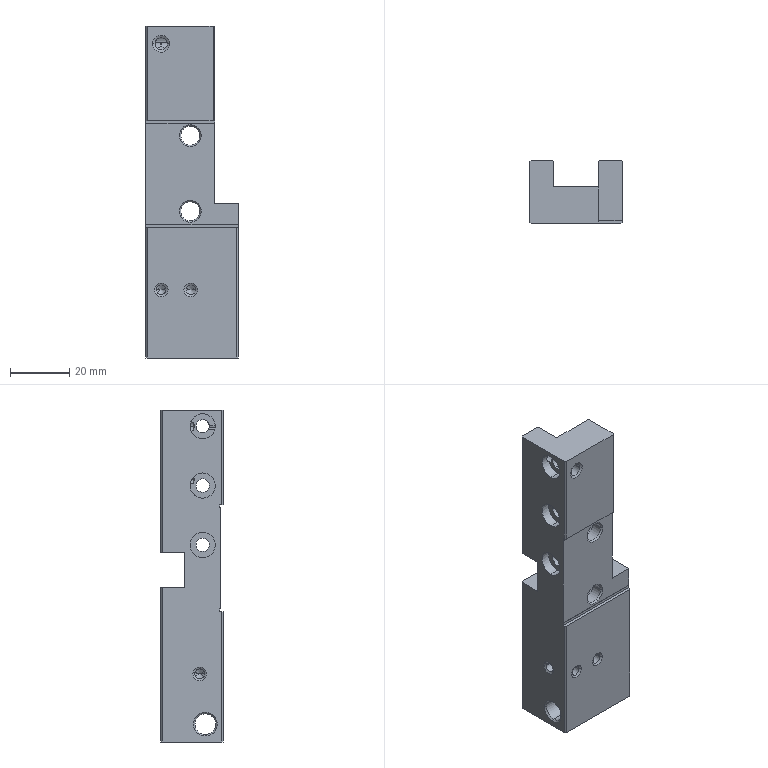Part | NX | 1 solid | 144 faces | box 31.2 x 21.2 x 112 mm | volume 41721 mm3 | cone 57 | cylinder 48 | plane 39 | commonest cylinder face diameters 3.3 x16 2.5 x8 4.5 x6 8.5 x6 6.4 x4 11 x4